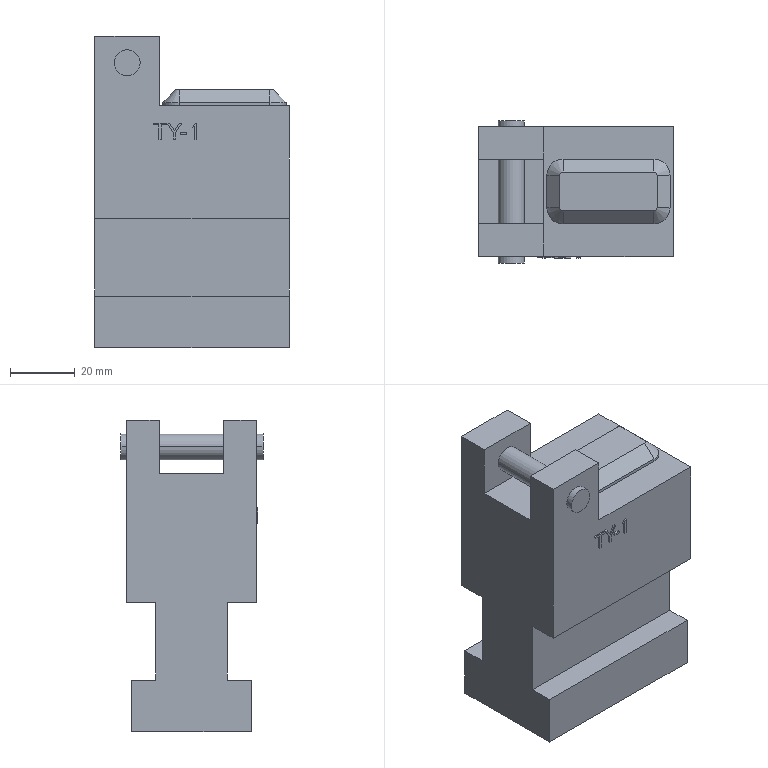Part | 1 solid | 77 faces | box 60 x 43.85 x 96.201 mm | volume 165060 mm3 | plane 61 | cylinder 10 | cone 4 | other 2 | commonest cylinder face diameters 8 x6 10 x4